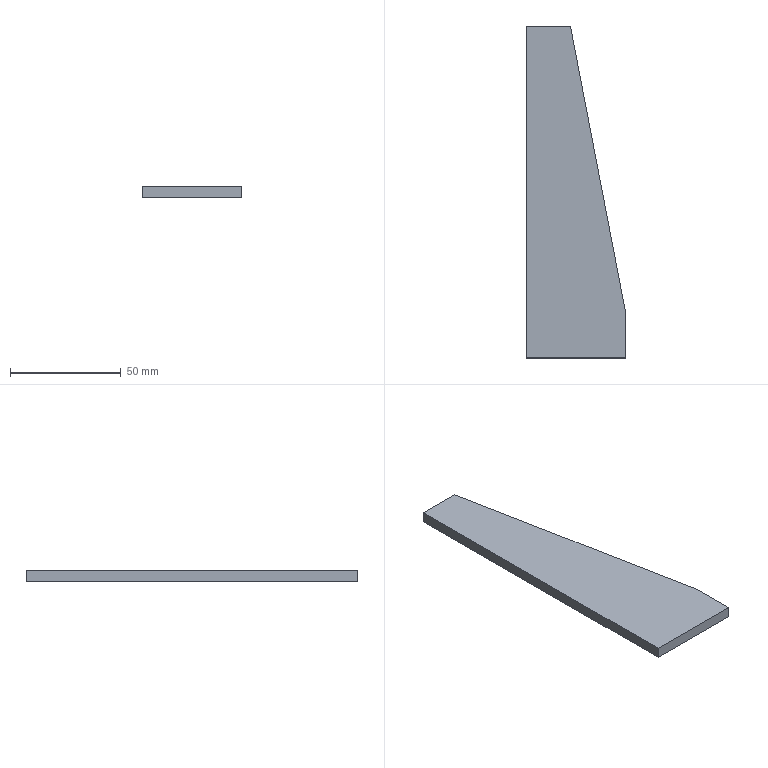Part | SolidWorks | features Extrusion 1 | 1 solid | 7 faces | box 45 x 150 x 5 mm | volume 25625 mm3 | plane 7
STEP:
#1=CARTESIAN_POINT('',(0.,0.,-2.5));
#2=VERTEX_POINT('',#1);
#3=CARTESIAN_POINT('',(45.,0.,-2.5));
#4=VERTEX_POINT('',#3);
#5=CARTESIAN_POINT('',(45.,0.,-2.5));
#6=DIRECTION('',(1.,0.,0.));
#7=VECTOR('',#6,1000.);
#8=LINE('',#5,#7);
#9=EDGE_CURVE('',#2,#4,#8,.T.);
#10=ORIENTED_EDGE('',*,*,#9,.T.);
#11=CARTESIAN_POINT('',(45.,0.,2.5));
#12=VERTEX_POINT('',#11);
#13=CARTESIAN_POINT('',(45.,0.,2.5));
#14=DIRECTION('',(0.,0.,-1.));
#15=VECTOR('',#14,1000.);
#16=LINE('',#13,#15);
#17=EDGE_CURVE('',#12,#4,#16,.T.);
#18=ORIENTED_EDGE('',*,*,#17,.F.);
#19=CARTESIAN_POINT('',(0.,0.,2.5));
#20=VERTEX_POINT('',#19);
#21=CARTESIAN_POINT('',(45.,0.,2.5));
#22=DIRECTION('',(1.,0.,0.));
#23=VECTOR('',#22,1000.);
#24=LINE('',#21,#23);
#25=EDGE_CURVE('',#20,#12,#24,.T.);
#26=ORIENTED_EDGE('',*,*,#25,.F.);
#27=CARTESIAN_POINT('',(0.,0.,2.5));
#28=DIRECTION('',(0.,0.,-1.));
#29=VECTOR('',#28,1000.);
#30=LINE('',#27,#29);
#31=EDGE_CURVE('',#20,#2,#30,.T.);
#32=ORIENTED_EDGE('',*,*,#31,.T.);
#33=EDGE_LOOP('',(#10,#18,#26,#32));
#34=FACE_OUTER_BOUND('',#33,.T.);
#35=CARTESIAN_POINT('',(45.,0.,2.5));
#36=DIRECTION('',(0.,1.,0.));
#37=DIRECTION('',(0.,0.,1.));
#38=AXIS2_PLACEMENT_3D('',#35,#36,#37);
#39=PLANE('',#38);
#40=ADVANCED_FACE('',(#34),#39,.F.);
#41=CARTESIAN_POINT('',(45.,20.,-2.5));
#42=VERTEX_POINT('',#41);
#43=CARTESIAN_POINT('',(45.,20.,-2.5));
#44=DIRECTION('',(0.,1.,0.));
#45=VECTOR('',#44,1000.);
#46=LINE('',#43,#45);
#47=EDGE_CURVE('',#4,#42,#46,.T.);
#48=ORIENTED_EDGE('',*,*,#47,.T.);
#49=CARTESIAN_POINT('',(45.,20.,2.5));
#50=VERTEX_POINT('',#49);
#51=CARTESIAN_POINT('',(45.,20.,2.5));
#52=DIRECTION('',(0.,0.,-1.));
#53=VECTOR('',#52,1000.);
#54=LINE('',#51,#53);
#55=EDGE_CURVE('',#50,#42,#54,.T.);
#56=ORIENTED_EDGE('',*,*,#55,.F.);
#57=CARTESIAN_POINT('',(45.,20.,2.5));
#58=DIRECTION('',(0.,1.,0.));
#59=VECTOR('',#58,1000.);
#60=LINE('',#57,#59);
#61=EDGE_CURVE('',#12,#50,#60,.T.);
#62=ORIENTED_EDGE('',*,*,#61,.F.);
#63=ORIENTED_EDGE('',*,*,#17,.T.);
#64=EDGE_LOOP('',(#48,#56,#62,#63));
#65=FACE_OUTER_BOUND('',#64,.T.);
#66=CARTESIAN_POINT('',(45.,20.,2.5));
#67=DIRECTION('',(-1.,0.,0.));
#68=DIRECTION('',(0.,0.,1.));
#69=AXIS2_PLACEMENT_3D('',#66,#67,#68);
#70=PLANE('',#69);
#71=ADVANCED_FACE('',(#65),#70,.F.);
#72=CARTESIAN_POINT('',(20.,150.,-2.5));
#73=VERTEX_POINT('',#72);
#74=CARTESIAN_POINT('',(20.,150.,-2.5));
#75=DIRECTION('',(-0.1888,0.982,0.));
#76=VECTOR('',#75,1000.);
#77=LINE('',#74,#76);
#78=EDGE_CURVE('',#42,#73,#77,.T.);
#79=ORIENTED_EDGE('',*,*,#78,.T.);
#80=CARTESIAN_POINT('',(20.,150.,2.5));
#81=VERTEX_POINT('',#80);
#82=CARTESIAN_POINT('',(20.,150.,2.5));
#83=DIRECTION('',(0.,0.,-1.));
#84=VECTOR('',#83,1000.);
#85=LINE('',#82,#84);
#86=EDGE_CURVE('',#81,#73,#85,.T.);
#87=ORIENTED_EDGE('',*,*,#86,.F.);
#88=CARTESIAN_POINT('',(20.,150.,2.5));
#89=DIRECTION('',(-0.1888,0.982,0.));
#90=VECTOR('',#89,1000.);
#91=LINE('',#88,#90);
#92=EDGE_CURVE('',#50,#81,#91,.T.);
#93=ORIENTED_EDGE('',*,*,#92,.F.);
#94=ORIENTED_EDGE('',*,*,#55,.T.);
#95=EDGE_LOOP('',(#79,#87,#93,#94));
#96=FACE_OUTER_BOUND('',#95,.T.);
#97=CARTESIAN_POINT('',(20.,150.,2.5));
#98=DIRECTION('',(-0.982,-0.1888,0.));
#99=DIRECTION('',(0.1888,-0.982,0.));
#100=AXIS2_PLACEMENT_3D('',#97,#98,#99);
#101=PLANE('',#100);
#102=ADVANCED_FACE('',(#96),#101,.F.);
#103=CARTESIAN_POINT('',(0.,150.,-2.5));
#104=VERTEX_POINT('',#103);
#105=CARTESIAN_POINT('',(0.,150.,-2.5));
#106=DIRECTION('',(-1.,0.,0.));
#107=VECTOR('',#106,1000.);
#108=LINE('',#105,#107);
#109=EDGE_CURVE('',#73,#104,#108,.T.);
#110=ORIENTED_EDGE('',*,*,#109,.T.);
#111=CARTESIAN_POINT('',(0.,150.,2.5));
#112=VERTEX_POINT('',#111);
#113=CARTESIAN_POINT('',(0.,150.,2.5));
#114=DIRECTION('',(0.,0.,-1.));
#115=VECTOR('',#114,1000.);
#116=LINE('',#113,#115);
#117=EDGE_CURVE('',#112,#104,#116,.T.);
#118=ORIENTED_EDGE('',*,*,#117,.F.);
#119=CARTESIAN_POINT('',(0.,150.,2.5));
#120=DIRECTION('',(-1.,0.,0.));
#121=VECTOR('',#120,1000.);
#122=LINE('',#119,#121);
#123=EDGE_CURVE('',#81,#112,#122,.T.);
#124=ORIENTED_EDGE('',*,*,#123,.F.);
#125=ORIENTED_EDGE('',*,*,#86,.T.);
#126=EDGE_LOOP('',(#110,#118,#124,#125));
#127=FACE_OUTER_BOUND('',#126,.T.);
#128=CARTESIAN_POINT('',(0.,150.,2.5));
#129=DIRECTION('',(0.,-1.,0.));
#130=DIRECTION('',(0.,0.,-1.));
#131=AXIS2_PLACEMENT_3D('',#128,#129,#130);
#132=PLANE('',#131);
#133=ADVANCED_FACE('',(#127),#132,.F.);
#134=CARTESIAN_POINT('',(0.,0.,-2.5));
#135=DIRECTION('',(0.,-1.,0.));
#136=VECTOR('',#135,1000.);
#137=LINE('',#134,#136);
#138=EDGE_CURVE('',#104,#2,#137,.T.);
#139=ORIENTED_EDGE('',*,*,#138,.T.);
#140=ORIENTED_EDGE('',*,*,#31,.F.);
#141=CARTESIAN_POINT('',(0.,0.,2.5));
#142=DIRECTION('',(0.,-1.,0.));
#143=VECTOR('',#142,1000.);
#144=LINE('',#141,#143);
#145=EDGE_CURVE('',#112,#20,#144,.T.);
#146=ORIENTED_EDGE('',*,*,#145,.F.);
#147=ORIENTED_EDGE('',*,*,#117,.T.);
#148=EDGE_LOOP('',(#139,#140,#146,#147));
#149=FACE_OUTER_BOUND('',#148,.T.);
#150=CARTESIAN_POINT('',(0.,0.,2.5));
#151=DIRECTION('',(1.,0.,0.));
#152=DIRECTION('',(0.,0.,-1.));
#153=AXIS2_PLACEMENT_3D('',#150,#151,#152);
#154=PLANE('',#153);
#155=ADVANCED_FACE('',(#149),#154,.F.);
#156=ORIENTED_EDGE('',*,*,#25,.T.);
#157=ORIENTED_EDGE('',*,*,#61,.T.);
#158=ORIENTED_EDGE('',*,*,#92,.T.);
#159=ORIENTED_EDGE('',*,*,#123,.T.);
#160=ORIENTED_EDGE('',*,*,#145,.T.);
#161=EDGE_LOOP('',(#156,#157,#158,#159,#160));
#162=FACE_OUTER_BOUND('',#161,.T.);
#163=CARTESIAN_POINT('',(0.,0.,2.5));
#164=DIRECTION('',(0.,0.,-1.));
#165=DIRECTION('',(-1.,0.,0.));
#166=AXIS2_PLACEMENT_3D('',#163,#164,#165);
#167=PLANE('',#166);
#168=ADVANCED_FACE('',(#162),#167,.F.);
#169=ORIENTED_EDGE('',*,*,#9,.F.);
#170=ORIENTED_EDGE('',*,*,#138,.F.);
#171=ORIENTED_EDGE('',*,*,#109,.F.);
#172=ORIENTED_EDGE('',*,*,#78,.F.);
#173=ORIENTED_EDGE('',*,*,#47,.F.);
#174=EDGE_LOOP('',(#169,#170,#171,#172,#173));
#175=FACE_OUTER_BOUND('',#174,.T.);
#176=CARTESIAN_POINT('',(0.,0.,-2.5));
#177=DIRECTION('',(0.,0.,-1.));
#178=DIRECTION('',(-1.,0.,0.));
#179=AXIS2_PLACEMENT_3D('',#176,#177,#178);
#180=PLANE('',#179);
#181=ADVANCED_FACE('',(#175),#180,.T.);
#182=CLOSED_SHELL('',(#40,#71,#102,#133,#155,#168,#181));
#183=MANIFOLD_SOLID_BREP('',#182);
#184=CARTESIAN_POINT('',(0.,0.,0.));
#185=DIRECTION('',(0.,0.,1.));
#186=DIRECTION('',(1.,0.,0.));
#187=AXIS2_PLACEMENT_3D('',#184,#185,#186);
#188=(LENGTH_UNIT()NAMED_UNIT(*)SI_UNIT(.MILLI.,.METRE.));
#189=UNCERTAINTY_MEASURE_WITH_UNIT(LENGTH_MEASURE(0.00001),#188,'','');
#190=(NAMED_UNIT(*)PLANE_ANGLE_UNIT()SI_UNIT($,.RADIAN.));
#191=(NAMED_UNIT(*)SI_UNIT($,.STERADIAN.)SOLID_ANGLE_UNIT());
#192=(GEOMETRIC_REPRESENTATION_CONTEXT(3)GLOBAL_UNCERTAINTY_ASSIGNED_CONTEXT((#189))GLOBAL_UNIT_ASSIGNED_CONTEXT((#188,#190,#191))REPRESENTATION_CONTEXT('',''));
#193=ADVANCED_BREP_SHAPE_REPRESENTATION('',(#183,#187),#192);